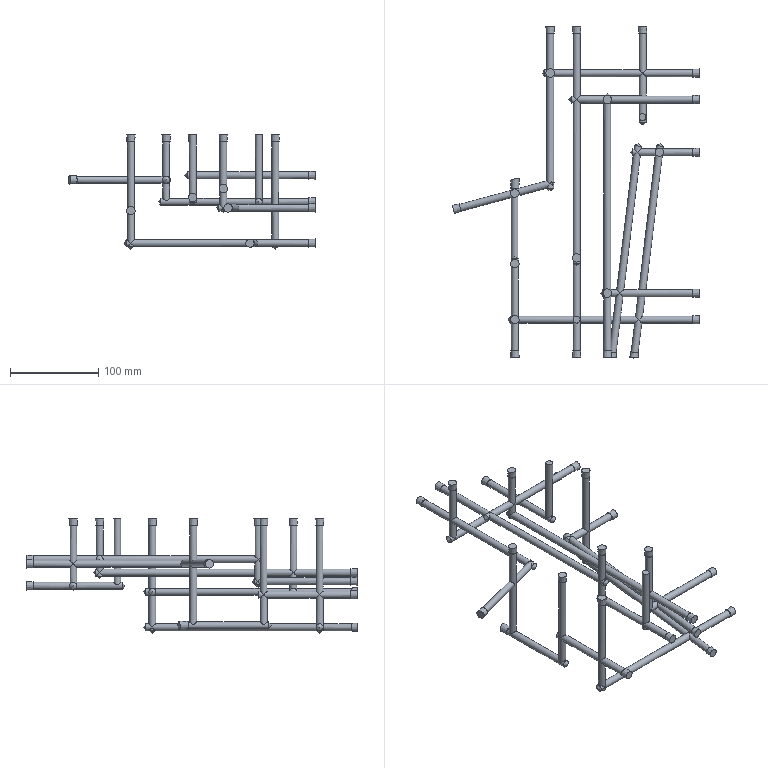Part | STEP file | 车灯-后视镜_id478_x_t | 1 solid | 167 faces | box 281.237 x 377 x 129.698 mm | volume 171076 mm3 | cylinder 64 | cone 55 | plane 48 | commonest cylinder face diameters 8 x64